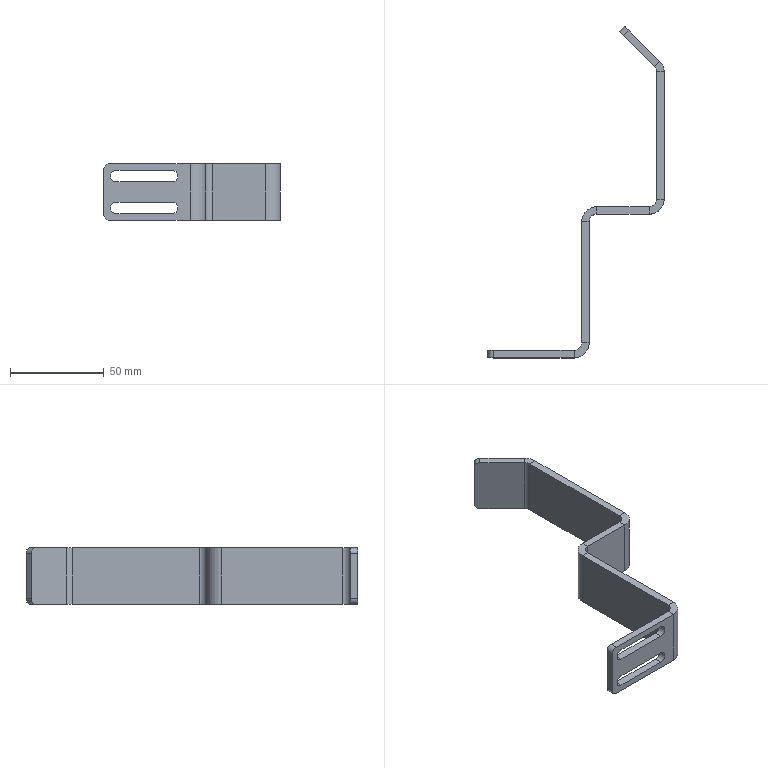Part | NX | features BREP 1 | 1 solid | 50 faces | box 94 x 176.828 x 30 mm | volume 30218 mm3 | plane 34 | cylinder 16 | commonest cylinder face diameters 6 x8 8 x4 16 x4
STEP:
#1=CARTESIAN_POINT('',(-32.,72.57,30.));
#2=VERTEX_POINT('',#1);
#3=CARTESIAN_POINT('',(-4.,72.57,30.));
#4=VERTEX_POINT('',#3);
#5=CARTESIAN_POINT('',(-75.773,72.57,30.));
#6=DIRECTION('',(1.,0.,0.));
#7=VECTOR('',#6,1000.);
#8=LINE('',#5,#7);
#9=EDGE_CURVE('',#2,#4,#8,.T.);
#10=ORIENTED_EDGE('',*,*,#9,.F.);
#11=CARTESIAN_POINT('',(-32.,72.57,0.));
#12=VERTEX_POINT('',#11);
#13=CARTESIAN_POINT('',(-32.,72.57,30.));
#14=DIRECTION('',(0.,0.,-1.));
#15=VECTOR('',#14,1000.);
#16=LINE('',#13,#15);
#17=EDGE_CURVE('',#2,#12,#16,.T.);
#18=ORIENTED_EDGE('',*,*,#17,.T.);
#19=CARTESIAN_POINT('',(-4.,72.57,0.));
#20=VERTEX_POINT('',#19);
#21=CARTESIAN_POINT('',(-75.773,72.57,0.));
#22=DIRECTION('',(1.,0.,0.));
#23=VECTOR('',#22,1000.);
#24=LINE('',#21,#23);
#25=EDGE_CURVE('',#12,#20,#24,.T.);
#26=ORIENTED_EDGE('',*,*,#25,.T.);
#27=CARTESIAN_POINT('',(-4.,72.57,30.));
#28=DIRECTION('',(0.,0.,-1.));
#29=VECTOR('',#28,1000.);
#30=LINE('',#27,#29);
#31=EDGE_CURVE('',#4,#20,#30,.T.);
#32=ORIENTED_EDGE('',*,*,#31,.F.);
#33=EDGE_LOOP('',(#10,#18,#26,#32));
#34=FACE_BOUND('',#33,.T.);
#35=CARTESIAN_POINT('',(-75.773,72.57,30.));
#36=DIRECTION('',(0.,1.,0.));
#37=DIRECTION('',(0.,0.,-1.));
#38=AXIS2_PLACEMENT_3D('',#35,#36,#37);
#39=PLANE('',#38);
#40=ADVANCED_FACE('',(#34),#39,.F.);
#41=CARTESIAN_POINT('',(-32.,76.57,30.));
#42=VERTEX_POINT('',#41);
#43=CARTESIAN_POINT('',(-32.,76.57,0.));
#44=VERTEX_POINT('',#43);
#45=CARTESIAN_POINT('',(-32.,76.57,30.));
#46=DIRECTION('',(0.,0.,-1.));
#47=VECTOR('',#46,1000.);
#48=LINE('',#45,#47);
#49=EDGE_CURVE('',#42,#44,#48,.T.);
#50=ORIENTED_EDGE('',*,*,#49,.F.);
#51=CARTESIAN_POINT('',(-4.,76.57,30.));
#52=VERTEX_POINT('',#51);
#53=CARTESIAN_POINT('',(-75.773,76.57,30.));
#54=DIRECTION('',(1.,0.,0.));
#55=VECTOR('',#54,1000.);
#56=LINE('',#53,#55);
#57=EDGE_CURVE('',#42,#52,#56,.T.);
#58=ORIENTED_EDGE('',*,*,#57,.T.);
#59=CARTESIAN_POINT('',(-4.,76.57,0.));
#60=VERTEX_POINT('',#59);
#61=CARTESIAN_POINT('',(-4.,76.57,30.));
#62=DIRECTION('',(0.,0.,-1.));
#63=VECTOR('',#62,1000.);
#64=LINE('',#61,#63);
#65=EDGE_CURVE('',#52,#60,#64,.T.);
#66=ORIENTED_EDGE('',*,*,#65,.T.);
#67=CARTESIAN_POINT('',(-75.773,76.57,0.));
#68=DIRECTION('',(1.,0.,0.));
#69=VECTOR('',#68,1000.);
#70=LINE('',#67,#69);
#71=EDGE_CURVE('',#44,#60,#70,.T.);
#72=ORIENTED_EDGE('',*,*,#71,.F.);
#73=EDGE_LOOP('',(#50,#58,#66,#72));
#74=FACE_BOUND('',#73,.T.);
#75=CARTESIAN_POINT('',(-75.773,76.57,30.));
#76=DIRECTION('',(0.,1.,0.));
#77=DIRECTION('',(0.,0.,-1.));
#78=AXIS2_PLACEMENT_3D('',#75,#76,#77);
#79=PLANE('',#78);
#80=ADVANCED_FACE('',(#74),#79,.T.);
#81=CARTESIAN_POINT('',(-32.,74.913,0.));
#82=DIRECTION('',(0.,-1.,0.));
#83=VECTOR('',#82,1000.);
#84=LINE('',#81,#83);
#85=EDGE_CURVE('',#44,#12,#84,.T.);
#86=ORIENTED_EDGE('',*,*,#85,.F.);
#87=ORIENTED_EDGE('',*,*,#71,.T.);
#88=CARTESIAN_POINT('',(-4.,74.913,0.));
#89=DIRECTION('',(0.,-1.,0.));
#90=VECTOR('',#89,1000.);
#91=LINE('',#88,#90);
#92=EDGE_CURVE('',#60,#20,#91,.T.);
#93=ORIENTED_EDGE('',*,*,#92,.T.);
#94=ORIENTED_EDGE('',*,*,#25,.F.);
#95=EDGE_LOOP('',(#86,#87,#93,#94));
#96=FACE_BOUND('',#95,.T.);
#97=CARTESIAN_POINT('',(78.227,74.913,0.));
#98=DIRECTION('',(0.,0.,-1.));
#99=DIRECTION('',(0.,-1.,0.));
#100=AXIS2_PLACEMENT_3D('',#97,#98,#99);
#101=PLANE('',#100);
#102=ADVANCED_FACE('',(#96),#101,.T.);
#103=CARTESIAN_POINT('',(-32.,80.57,30.));
#104=DIRECTION('',(0.,1.,0.));
#105=VECTOR('',#104,1000.);
#106=LINE('',#103,#105);
#107=EDGE_CURVE('',#2,#42,#106,.T.);
#108=ORIENTED_EDGE('',*,*,#107,.F.);
#109=ORIENTED_EDGE('',*,*,#9,.T.);
#110=CARTESIAN_POINT('',(-4.,80.57,30.));
#111=DIRECTION('',(0.,1.,0.));
#112=VECTOR('',#111,1000.);
#113=LINE('',#110,#112);
#114=EDGE_CURVE('',#4,#52,#113,.T.);
#115=ORIENTED_EDGE('',*,*,#114,.T.);
#116=ORIENTED_EDGE('',*,*,#57,.F.);
#117=EDGE_LOOP('',(#108,#109,#115,#116));
#118=FACE_BOUND('',#117,.T.);
#119=CARTESIAN_POINT('',(-79.773,80.57,30.));
#120=DIRECTION('',(0.,0.,1.));
#121=DIRECTION('',(0.,1.,0.));
#122=AXIS2_PLACEMENT_3D('',#119,#120,#121);
#123=PLANE('',#122);
#124=ADVANCED_FACE('',(#118),#123,.T.);
#125=CARTESIAN_POINT('',(-17.172,172.828,27.));
#126=VERTEX_POINT('',#125);
#127=CARTESIAN_POINT('',(-17.172,172.828,3.));
#128=VERTEX_POINT('',#127);
#129=CARTESIAN_POINT('',(-17.172,172.828,30.));
#130=DIRECTION('',(0.,0.,-1.));
#131=VECTOR('',#130,1000.);
#132=LINE('',#129,#131);
#133=EDGE_CURVE('',#126,#128,#132,.T.);
#134=ORIENTED_EDGE('',*,*,#133,.T.);
#135=CARTESIAN_POINT('',(-20.,170.,3.));
#136=VERTEX_POINT('',#135);
#137=CARTESIAN_POINT('',(-20.,170.,3.));
#138=DIRECTION('',(-0.7071,-0.7071,0.));
#139=VECTOR('',#138,1000.);
#140=LINE('',#137,#139);
#141=EDGE_CURVE('',#128,#136,#140,.T.);
#142=ORIENTED_EDGE('',*,*,#141,.T.);
#143=CARTESIAN_POINT('',(-20.,170.,27.));
#144=VERTEX_POINT('',#143);
#145=CARTESIAN_POINT('',(-20.,170.,30.));
#146=DIRECTION('',(0.,0.,-1.));
#147=VECTOR('',#146,1000.);
#148=LINE('',#145,#147);
#149=EDGE_CURVE('',#144,#136,#148,.T.);
#150=ORIENTED_EDGE('',*,*,#149,.F.);
#151=CARTESIAN_POINT('',(-20.,170.,27.));
#152=DIRECTION('',(0.7071,0.7071,0.));
#153=VECTOR('',#152,1000.);
#154=LINE('',#151,#153);
#155=EDGE_CURVE('',#144,#126,#154,.T.);
#156=ORIENTED_EDGE('',*,*,#155,.T.);
#157=EDGE_LOOP('',(#134,#142,#150,#156));
#158=FACE_BOUND('',#157,.T.);
#159=CARTESIAN_POINT('',(-20.,170.,30.));
#160=DIRECTION('',(-0.7071,0.7071,0.));
#161=DIRECTION('',(0.7071,0.7071,0.));
#162=AXIS2_PLACEMENT_3D('',#159,#160,#161);
#163=PLANE('',#162);
#164=ADVANCED_FACE('',(#158),#163,.T.);
#165=CARTESIAN_POINT('',(-1.172,151.172,0.));
#166=VERTEX_POINT('',#165);
#167=CARTESIAN_POINT('',(-17.879,167.879,0.));
#168=VERTEX_POINT('',#167);
#169=CARTESIAN_POINT('',(0.,150.,0.));
#170=DIRECTION('',(-0.7071,0.7071,0.));
#171=VECTOR('',#170,1000.);
#172=LINE('',#169,#171);
#173=EDGE_CURVE('',#166,#168,#172,.T.);
#174=ORIENTED_EDGE('',*,*,#173,.T.);
#175=CARTESIAN_POINT('',(-15.05,170.707,0.));
#176=VERTEX_POINT('',#175);
#177=CARTESIAN_POINT('',(-20.707,165.05,0.));
#178=DIRECTION('',(0.7071,0.7071,0.));
#179=VECTOR('',#178,1000.);
#180=LINE('',#177,#179);
#181=EDGE_CURVE('',#168,#176,#180,.T.);
#182=ORIENTED_EDGE('',*,*,#181,.T.);
#183=CARTESIAN_POINT('',(1.657,154.,0.));
#184=VERTEX_POINT('',#183);
#185=CARTESIAN_POINT('',(2.828,152.828,0.));
#186=DIRECTION('',(-0.7071,0.7071,0.));
#187=VECTOR('',#186,1000.);
#188=LINE('',#185,#187);
#189=EDGE_CURVE('',#184,#176,#188,.T.);
#190=ORIENTED_EDGE('',*,*,#189,.F.);
#191=CARTESIAN_POINT('',(1.657,154.,0.));
#192=DIRECTION('',(-0.7071,-0.7071,0.));
#193=VECTOR('',#192,1000.);
#194=LINE('',#191,#193);
#195=EDGE_CURVE('',#184,#166,#194,.T.);
#196=ORIENTED_EDGE('',*,*,#195,.T.);
#197=EDGE_LOOP('',(#174,#182,#190,#196));
#198=FACE_BOUND('',#197,.T.);
#199=CARTESIAN_POINT('',(-4.,148.343,0.));
#200=DIRECTION('',(0.,0.,-1.));
#201=DIRECTION('',(1.,0.,0.));
#202=AXIS2_PLACEMENT_3D('',#199,#200,#201);
#203=PLANE('',#202);
#204=ADVANCED_FACE('',(#198),#203,.T.);
#205=ORIENTED_EDGE('',*,*,#189,.T.);
#206=CARTESIAN_POINT('',(-15.05,170.707,3.));
#207=DIRECTION('',(0.7071,0.7071,0.));
#208=DIRECTION('',(0.7071,-0.7071,0.));
#209=AXIS2_PLACEMENT_3D('',#206,#207,#208);
#210=CIRCLE('',#209,3.);
#211=EDGE_CURVE('',#176,#128,#210,.T.);
#212=ORIENTED_EDGE('',*,*,#211,.T.);
#213=ORIENTED_EDGE('',*,*,#133,.F.);
#214=CARTESIAN_POINT('',(-15.05,170.707,30.));
#215=VERTEX_POINT('',#214);
#216=CARTESIAN_POINT('',(-15.05,170.707,27.));
#217=DIRECTION('',(0.7071,0.7071,0.));
#218=DIRECTION('',(0.7071,-0.7071,0.));
#219=AXIS2_PLACEMENT_3D('',#216,#217,#218);
#220=CIRCLE('',#219,3.);
#221=EDGE_CURVE('',#126,#215,#220,.T.);
#222=ORIENTED_EDGE('',*,*,#221,.T.);
#223=CARTESIAN_POINT('',(1.657,154.,30.));
#224=VERTEX_POINT('',#223);
#225=CARTESIAN_POINT('',(2.828,152.828,30.));
#226=DIRECTION('',(-0.7071,0.7071,0.));
#227=VECTOR('',#226,1000.);
#228=LINE('',#225,#227);
#229=EDGE_CURVE('',#224,#215,#228,.T.);
#230=ORIENTED_EDGE('',*,*,#229,.F.);
#231=CARTESIAN_POINT('',(1.657,154.,30.));
#232=DIRECTION('',(0.,0.,-1.));
#233=VECTOR('',#232,1000.);
#234=LINE('',#231,#233);
#235=EDGE_CURVE('',#224,#184,#234,.T.);
#236=ORIENTED_EDGE('',*,*,#235,.T.);
#237=EDGE_LOOP('',(#205,#212,#213,#222,#230,#236));
#238=FACE_BOUND('',#237,.T.);
#239=CARTESIAN_POINT('',(2.828,152.828,30.));
#240=DIRECTION('',(-0.7071,-0.7071,0.));
#241=DIRECTION('',(-0.7071,0.7071,0.));
#242=AXIS2_PLACEMENT_3D('',#239,#240,#241);
#243=PLANE('',#242);
#244=ADVANCED_FACE('',(#238),#243,.F.);
#245=ORIENTED_EDGE('',*,*,#229,.T.);
#246=CARTESIAN_POINT('',(-17.879,167.879,30.));
#247=VERTEX_POINT('',#246);
#248=CARTESIAN_POINT('',(-16.707,169.05,30.));
#249=DIRECTION('',(-0.7071,-0.7071,0.));
#250=VECTOR('',#249,1000.);
#251=LINE('',#248,#250);
#252=EDGE_CURVE('',#215,#247,#251,.T.);
#253=ORIENTED_EDGE('',*,*,#252,.T.);
#254=CARTESIAN_POINT('',(-1.172,151.172,30.));
#255=VERTEX_POINT('',#254);
#256=CARTESIAN_POINT('',(0.,150.,30.));
#257=DIRECTION('',(-0.7071,0.7071,0.));
#258=VECTOR('',#257,1000.);
#259=LINE('',#256,#258);
#260=EDGE_CURVE('',#255,#247,#259,.T.);
#261=ORIENTED_EDGE('',*,*,#260,.F.);
#262=CARTESIAN_POINT('',(-1.172,151.172,30.));
#263=DIRECTION('',(0.7071,0.7071,0.));
#264=VECTOR('',#263,1000.);
#265=LINE('',#262,#264);
#266=EDGE_CURVE('',#255,#224,#265,.T.);
#267=ORIENTED_EDGE('',*,*,#266,.T.);
#268=EDGE_LOOP('',(#245,#253,#261,#267));
#269=FACE_BOUND('',#268,.T.);
#270=CARTESIAN_POINT('',(4.,148.343,30.));
#271=DIRECTION('',(0.,0.,1.));
#272=DIRECTION('',(-1.,0.,0.));
#273=AXIS2_PLACEMENT_3D('',#270,#271,#272);
#274=PLANE('',#273);
#275=ADVANCED_FACE('',(#269),#274,.T.);
#276=ORIENTED_EDGE('',*,*,#149,.T.);
#277=CARTESIAN_POINT('',(-17.879,167.879,3.));
#278=DIRECTION('',(-0.7071,-0.7071,0.));
#279=DIRECTION('',(0.7071,-0.7071,0.));
#280=AXIS2_PLACEMENT_3D('',#277,#278,#279);
#281=CIRCLE('',#280,3.);
#282=EDGE_CURVE('',#136,#168,#281,.T.);
#283=ORIENTED_EDGE('',*,*,#282,.T.);
#284=ORIENTED_EDGE('',*,*,#173,.F.);
#285=CARTESIAN_POINT('',(-1.172,151.172,30.));
#286=DIRECTION('',(0.,0.,-1.));
#287=VECTOR('',#286,1000.);
#288=LINE('',#285,#287);
#289=EDGE_CURVE('',#255,#166,#288,.T.);
#290=ORIENTED_EDGE('',*,*,#289,.F.);
#291=ORIENTED_EDGE('',*,*,#260,.T.);
#292=CARTESIAN_POINT('',(-17.879,167.879,27.));
#293=DIRECTION('',(-0.7071,-0.7071,0.));
#294=DIRECTION('',(0.7071,-0.7071,0.));
#295=AXIS2_PLACEMENT_3D('',#292,#293,#294);
#296=CIRCLE('',#295,3.);
#297=EDGE_CURVE('',#247,#144,#296,.T.);
#298=ORIENTED_EDGE('',*,*,#297,.T.);
#299=EDGE_LOOP('',(#276,#283,#284,#290,#291,#298));
#300=FACE_BOUND('',#299,.T.);
#301=CARTESIAN_POINT('',(0.,150.,30.));
#302=DIRECTION('',(-0.7071,-0.7071,0.));
#303=DIRECTION('',(-0.7071,0.7071,0.));
#304=AXIS2_PLACEMENT_3D('',#301,#302,#303);
#305=PLANE('',#304);
#306=ADVANCED_FACE('',(#300),#305,.T.);
#307=CARTESIAN_POINT('',(0.,148.343,0.));
#308=VERTEX_POINT('',#307);
#309=CARTESIAN_POINT('',(4.,148.343,0.));
#310=VERTEX_POINT('',#309);
#311=CARTESIAN_POINT('',(0.,148.343,0.));
#312=DIRECTION('',(1.,0.,0.));
#313=VECTOR('',#312,1000.);
#314=LINE('',#311,#313);
#315=EDGE_CURVE('',#308,#310,#314,.T.);
#316=ORIENTED_EDGE('',*,*,#315,.F.);
#317=CARTESIAN_POINT('',(-4.,148.343,0.));
#318=DIRECTION('',(0.,0.,1.));
#319=DIRECTION('',(-1.,0.,0.));
#320=AXIS2_PLACEMENT_3D('',#317,#318,#319);
#321=CIRCLE('',#320,4.);
#322=EDGE_CURVE('',#308,#166,#321,.T.);
#323=ORIENTED_EDGE('',*,*,#322,.T.);
#324=ORIENTED_EDGE('',*,*,#195,.F.);
#325=CARTESIAN_POINT('',(-4.,148.343,0.));
#326=DIRECTION('',(0.,0.,1.));
#327=DIRECTION('',(1.,0.,0.));
#328=AXIS2_PLACEMENT_3D('',#325,#326,#327);
#329=CIRCLE('',#328,8.);
#330=EDGE_CURVE('',#310,#184,#329,.T.);
#331=ORIENTED_EDGE('',*,*,#330,.F.);
#332=EDGE_LOOP('',(#316,#323,#324,#331));
#333=FACE_BOUND('',#332,.T.);
#334=CARTESIAN_POINT('',(0.,148.343,0.));
#335=DIRECTION('',(0.,0.,-1.));
#336=DIRECTION('',(1.,0.,0.));
#337=AXIS2_PLACEMENT_3D('',#334,#335,#336);
#338=PLANE('',#337);
#339=ADVANCED_FACE('',(#333),#338,.T.);
#340=ORIENTED_EDGE('',*,*,#330,.T.);
#341=ORIENTED_EDGE('',*,*,#235,.F.);
#342=CARTESIAN_POINT('',(4.,148.343,30.));
#343=VERTEX_POINT('',#342);
#344=CARTESIAN_POINT('',(-4.,148.343,30.));
#345=DIRECTION('',(0.,0.,1.));
#346=DIRECTION('',(1.,0.,0.));
#347=AXIS2_PLACEMENT_3D('',#344,#345,#346);
#348=CIRCLE('',#347,8.);
#349=EDGE_CURVE('',#343,#224,#348,.T.);
#350=ORIENTED_EDGE('',*,*,#349,.F.);
#351=CARTESIAN_POINT('',(4.,148.343,30.));
#352=DIRECTION('',(0.,0.,-1.));
#353=VECTOR('',#352,1000.);
#354=LINE('',#351,#353);
#355=EDGE_CURVE('',#343,#310,#354,.T.);
#356=ORIENTED_EDGE('',*,*,#355,.T.);
#357=EDGE_LOOP('',(#340,#341,#350,#356));
#358=FACE_BOUND('',#357,.T.);
#359=CARTESIAN_POINT('',(-4.,148.343,30.));
#360=DIRECTION('',(0.,0.,-1.));
#361=DIRECTION('',(1.,0.,0.));
#362=AXIS2_PLACEMENT_3D('',#359,#360,#361);
#363=CYLINDRICAL_SURFACE('',#362,8.);
#364=ADVANCED_FACE('',(#358),#363,.T.);
#365=ORIENTED_EDGE('',*,*,#266,.F.);
#366=CARTESIAN_POINT('',(0.,148.343,30.));
#367=VERTEX_POINT('',#366);
#368=CARTESIAN_POINT('',(-4.,148.343,30.));
#369=DIRECTION('',(0.,0.,1.));
#370=DIRECTION('',(-1.,0.,0.));
#371=AXIS2_PLACEMENT_3D('',#368,#369,#370);
#372=CIRCLE('',#371,4.);
#373=EDGE_CURVE('',#367,#255,#372,.T.);
#374=ORIENTED_EDGE('',*,*,#373,.F.);
#375=CARTESIAN_POINT('',(4.,148.343,30.));
#376=DIRECTION('',(-1.,0.,0.));
#377=VECTOR('',#376,1000.);
#378=LINE('',#375,#377);
#379=EDGE_CURVE('',#343,#367,#378,.T.);
#380=ORIENTED_EDGE('',*,*,#379,.F.);
#381=ORIENTED_EDGE('',*,*,#349,.T.);
#382=EDGE_LOOP('',(#365,#374,#380,#381));
#383=FACE_BOUND('',#382,.T.);
#384=CARTESIAN_POINT('',(-1.172,151.172,30.));
#385=DIRECTION('',(0.,0.,1.));
#386=DIRECTION('',(-1.,0.,0.));
#387=AXIS2_PLACEMENT_3D('',#384,#385,#386);
#388=PLANE('',#387);
#389=ADVANCED_FACE('',(#383),#388,.T.);
#390=ORIENTED_EDGE('',*,*,#322,.F.);
#391=CARTESIAN_POINT('',(0.,148.343,30.));
#392=DIRECTION('',(0.,0.,-1.));
#393=VECTOR('',#392,1000.);
#394=LINE('',#391,#393);
#395=EDGE_CURVE('',#367,#308,#394,.T.);
#396=ORIENTED_EDGE('',*,*,#395,.F.);
#397=ORIENTED_EDGE('',*,*,#373,.T.);
#398=ORIENTED_EDGE('',*,*,#289,.T.);
#399=EDGE_LOOP('',(#390,#396,#397,#398));
#400=FACE_BOUND('',#399,.T.);
#401=CARTESIAN_POINT('',(-4.,148.343,30.));
#402=DIRECTION('',(0.,0.,-1.));
#403=DIRECTION('',(1.,0.,0.));
#404=AXIS2_PLACEMENT_3D('',#401,#402,#403);
#405=CYLINDRICAL_SURFACE('',#404,4.);
#406=ADVANCED_FACE('',(#400),#405,.F.);
#407=CARTESIAN_POINT('',(0.,80.57,30.));
#408=VERTEX_POINT('',#407);
#409=CARTESIAN_POINT('',(0.,80.57,0.));
#410=VERTEX_POINT('',#409);
#411=CARTESIAN_POINT('',(0.,80.57,30.));
#412=DIRECTION('',(0.,0.,-1.));
#413=VECTOR('',#412,1000.);
#414=LINE('',#411,#413);
#415=EDGE_CURVE('',#408,#410,#414,.T.);
#416=ORIENTED_EDGE('',*,*,#415,.F.);
#417=CARTESIAN_POINT('',(0.,0.,30.));
#418=DIRECTION('',(0.,1.,0.));
#419=VECTOR('',#418,1000.);
#420=LINE('',#417,#419);
#421=EDGE_CURVE('',#408,#367,#420,.T.);
#422=ORIENTED_EDGE('',*,*,#421,.T.);
#423=ORIENTED_EDGE('',*,*,#395,.T.);
#424=CARTESIAN_POINT('',(0.,0.,0.));
#425=DIRECTION('',(0.,1.,0.));
#426=VECTOR('',#425,1000.);
#427=LINE('',#424,#426);
#428=EDGE_CURVE('',#410,#308,#427,.T.);
#429=ORIENTED_EDGE('',*,*,#428,.F.);
#430=EDGE_LOOP('',(#416,#422,#423,#429));
#431=FACE_BOUND('',#430,.T.);
#432=CARTESIAN_POINT('',(0.,0.,30.));
#433=DIRECTION('',(-1.,0.,0.));
#434=DIRECTION('',(0.,0.,-1.));
#435=AXIS2_PLACEMENT_3D('',#432,#433,#434);
#436=PLANE('',#435);
#437=ADVANCED_FACE('',(#431),#436,.T.);
#438=CARTESIAN_POINT('',(4.,80.57,30.));
#439=VERTEX_POINT('',#438);
#440=CARTESIAN_POINT('',(-4.,80.57,30.));
#441=DIRECTION('',(-1.,0.,0.));
#442=VECTOR('',#441,1000.);
#443=LINE('',#440,#442);
#444=EDGE_CURVE('',#439,#408,#443,.T.);
#445=ORIENTED_EDGE('',*,*,#444,.F.);
#446=CARTESIAN_POINT('',(4.,0.,30.));
#447=DIRECTION('',(0.,1.,0.));
#448=VECTOR('',#447,1000.);
#449=LINE('',#446,#448);
#450=EDGE_CURVE('',#439,#343,#449,.T.);
#451=ORIENTED_EDGE('',*,*,#450,.T.);
#452=ORIENTED_EDGE('',*,*,#379,.T.);
#453=ORIENTED_EDGE('',*,*,#421,.F.);
#454=EDGE_LOOP('',(#445,#451,#452,#453));
#455=FACE_BOUND('',#454,.T.);
#456=CARTESIAN_POINT('',(-4.,-4.,30.));
#457=DIRECTION('',(0.,0.,1.));
#458=DIRECTION('',(-1.,0.,0.));
#459=AXIS2_PLACEMENT_3D('',#456,#457,#458);
#460=PLANE('',#459);
#461=ADVANCED_FACE('',(#455),#460,.T.);
#462=ORIENTED_EDGE('',*,*,#450,.F.);
#463=CARTESIAN_POINT('',(4.,80.57,0.));
#464=VERTEX_POINT('',#463);
#465=CARTESIAN_POINT('',(4.,80.57,30.));
#466=DIRECTION('',(0.,0.,-1.));
#467=VECTOR('',#466,1000.);
#468=LINE('',#465,#467);
#469=EDGE_CURVE('',#439,#464,#468,.T.);
#470=ORIENTED_EDGE('',*,*,#469,.T.);
#471=CARTESIAN_POINT('',(4.,0.,0.));
#472=DIRECTION('',(0.,1.,0.));
#473=VECTOR('',#472,1000.);
#474=LINE('',#471,#473);
#475=EDGE_CURVE('',#464,#310,#474,.T.);
#476=ORIENTED_EDGE('',*,*,#475,.T.);
#477=ORIENTED_EDGE('',*,*,#355,.F.);
#478=EDGE_LOOP('',(#462,#470,#476,#477));
#479=FACE_BOUND('',#478,.T.);
#480=CARTESIAN_POINT('',(4.,0.,30.));
#481=DIRECTION('',(-1.,0.,0.));
#482=DIRECTION('',(0.,0.,-1.));
#483=AXIS2_PLACEMENT_3D('',#480,#481,#482);
#484=PLANE('',#483);
#485=ADVANCED_FACE('',(#479),#484,.F.);
#486=CARTESIAN_POINT('',(1.657,80.57,0.));
#487=DIRECTION('',(1.,0.,0.));
#488=VECTOR('',#487,1000.);
#489=LINE('',#486,#488);
#490=EDGE_CURVE('',#410,#464,#489,.T.);
#491=ORIENTED_EDGE('',*,*,#490,.F.);
#492=ORIENTED_EDGE('',*,*,#428,.T.);
#493=ORIENTED_EDGE('',*,*,#315,.T.);
#494=ORIENTED_EDGE('',*,*,#475,.F.);
#495=EDGE_LOOP('',(#491,#492,#493,#494));
#496=FACE_BOUND('',#495,.T.);
#497=CARTESIAN_POINT('',(1.657,154.,0.));
#498=DIRECTION('',(0.,0.,-1.));
#499=DIRECTION('',(1.,0.,0.));
#500=AXIS2_PLACEMENT_3D('',#497,#498,#499);
#501=PLANE('',#500);
#502=ADVANCED_FACE('',(#496),#501,.T.);
#503=ORIENTED_EDGE('',*,*,#114,.F.);
#504=CARTESIAN_POINT('',(-4.,80.57,30.));
#505=DIRECTION('',(0.,0.,1.));
#506=DIRECTION('',(1.,0.,0.));
#507=AXIS2_PLACEMENT_3D('',#504,#505,#506);
#508=CIRCLE('',#507,8.);
#509=EDGE_CURVE('',#4,#439,#508,.T.);
#510=ORIENTED_EDGE('',*,*,#509,.T.);
#511=ORIENTED_EDGE('',*,*,#444,.T.);
#512=CARTESIAN_POINT('',(-4.,80.57,30.));
#513=DIRECTION('',(0.,0.,1.));
#514=DIRECTION('',(1.,0.,0.));
#515=AXIS2_PLACEMENT_3D('',#512,#513,#514);
#516=CIRCLE('',#515,4.);
#517=EDGE_CURVE('',#52,#408,#516,.T.);
#518=ORIENTED_EDGE('',*,*,#517,.F.);
#519=EDGE_LOOP('',(#503,#510,#511,#518));
#520=FACE_BOUND('',#519,.T.);
#521=CARTESIAN_POINT('',(-4.,80.57,30.));
#522=DIRECTION('',(0.,0.,-1.));
#523=DIRECTION('',(1.,0.,0.));
#524=AXIS2_PLACEMENT_3D('',#521,#522,#523);
#525=PLANE('',#524);
#526=ADVANCED_FACE('',(#520),#525,.F.);
#527=CARTESIAN_POINT('',(-4.,80.57,0.));
#528=DIRECTION('',(0.,0.,-1.));
#529=DIRECTION('',(1.,0.,0.));
#530=AXIS2_PLACEMENT_3D('',#527,#528,#529);
#531=CIRCLE('',#530,8.);
#532=EDGE_CURVE('',#464,#20,#531,.T.);
#533=ORIENTED_EDGE('',*,*,#532,.T.);
#534=ORIENTED_EDGE('',*,*,#92,.F.);
#535=CARTESIAN_POINT('',(-4.,80.57,0.));
#536=DIRECTION('',(0.,0.,-1.));
#537=DIRECTION('',(1.,0.,0.));
#538=AXIS2_PLACEMENT_3D('',#535,#536,#537);
#539=CIRCLE('',#538,4.);
#540=EDGE_CURVE('',#410,#60,#539,.T.);
#541=ORIENTED_EDGE('',*,*,#540,.F.);
#542=ORIENTED_EDGE('',*,*,#490,.T.);
#543=EDGE_LOOP('',(#533,#534,#541,#542));
#544=FACE_BOUND('',#543,.T.);
#545=CARTESIAN_POINT('',(-4.,80.57,0.));
#546=DIRECTION('',(0.,0.,1.));
#547=DIRECTION('',(-1.,0.,0.));
#548=AXIS2_PLACEMENT_3D('',#545,#546,#547);
#549=PLANE('',#548);
#550=ADVANCED_FACE('',(#544),#549,.F.);
#551=ORIENTED_EDGE('',*,*,#415,.T.);
#552=ORIENTED_EDGE('',*,*,#540,.T.);
#553=ORIENTED_EDGE('',*,*,#65,.F.);
#554=ORIENTED_EDGE('',*,*,#517,.T.);
#555=EDGE_LOOP('',(#551,#552,#553,#554));
#556=FACE_BOUND('',#555,.T.);
#557=CARTESIAN_POINT('',(-4.,80.57,-16.518));
#558=DIRECTION('',(0.,0.,1.));
#559=DIRECTION('',(-1.,0.,0.));
#560=AXIS2_PLACEMENT_3D('',#557,#558,#559);
#561=CYLINDRICAL_SURFACE('',#560,4.);
#562=ADVANCED_FACE('',(#556),#561,.F.);
#563=ORIENTED_EDGE('',*,*,#469,.F.);
#564=ORIENTED_EDGE('',*,*,#509,.F.);
#565=ORIENTED_EDGE('',*,*,#31,.T.);
#566=ORIENTED_EDGE('',*,*,#532,.F.);
#567=EDGE_LOOP('',(#563,#564,#565,#566));
#568=FACE_BOUND('',#567,.T.);
#569=CARTESIAN_POINT('',(-4.,80.57,-16.518));
#570=DIRECTION('',(0.,0.,1.));
#571=DIRECTION('',(-1.,0.,0.));
#572=AXIS2_PLACEMENT_3D('',#569,#570,#571);
#573=CYLINDRICAL_SURFACE('',#572,8.);
#574=ADVANCED_FACE('',(#568),#573,.T.);
#575=CARTESIAN_POINT('',(-36.,68.57,30.));
#576=VERTEX_POINT('',#575);
#577=CARTESIAN_POINT('',(-40.,68.57,30.));
#578=VERTEX_POINT('',#577);
#579=CARTESIAN_POINT('',(-44.,68.57,30.));
#580=DIRECTION('',(-1.,0.,0.));
#581=VECTOR('',#580,1000.);
#582=LINE('',#579,#581);
#583=EDGE_CURVE('',#576,#578,#582,.T.);
#584=ORIENTED_EDGE('',*,*,#583,.F.);
#585=CARTESIAN_POINT('',(-32.,68.57,30.));
#586=DIRECTION('',(0.,0.,-1.));
#587=DIRECTION('',(1.,0.,0.));
#588=AXIS2_PLACEMENT_3D('',#585,#586,#587);
#589=CIRCLE('',#588,4.);
#590=EDGE_CURVE('',#576,#2,#589,.T.);
#591=ORIENTED_EDGE('',*,*,#590,.T.);
#592=ORIENTED_EDGE('',*,*,#107,.T.);
#593=CARTESIAN_POINT('',(-32.,68.57,30.));
#594=DIRECTION('',(0.,0.,-1.));
#595=DIRECTION('',(-1.,0.,0.));
#596=AXIS2_PLACEMENT_3D('',#593,#594,#595);
#597=CIRCLE('',#596,8.);
#598=EDGE_CURVE('',#578,#42,#597,.T.);
#599=ORIENTED_EDGE('',*,*,#598,.F.);
#600=EDGE_LOOP('',(#584,#591,#592,#599));
#601=FACE_BOUND('',#600,.T.);
#602=CARTESIAN_POINT('',(-32.,68.57,30.));
#603=DIRECTION('',(0.,0.,1.));
#604=DIRECTION('',(-1.,0.,0.));
#605=AXIS2_PLACEMENT_3D('',#602,#603,#604);
#606=PLANE('',#605);
#607=ADVANCED_FACE('',(#601),#606,.T.);
#608=CARTESIAN_POINT('',(-36.,68.57,0.));
#609=VERTEX_POINT('',#608);
#610=CARTESIAN_POINT('',(-32.,68.57,0.));
#611=DIRECTION('',(0.,0.,1.));
#612=DIRECTION('',(1.,0.,0.));
#613=AXIS2_PLACEMENT_3D('',#610,#611,#612);
#614=CIRCLE('',#613,4.);
#615=EDGE_CURVE('',#12,#609,#614,.T.);
#616=ORIENTED_EDGE('',*,*,#615,.T.);
#617=CARTESIAN_POINT('',(-40.,68.57,0.));
#618=VERTEX_POINT('',#617);
#619=CARTESIAN_POINT('',(-38.343,68.57,0.));
#620=DIRECTION('',(1.,0.,0.));
#621=VECTOR('',#620,1000.);
#622=LINE('',#619,#621);
#623=EDGE_CURVE('',#618,#609,#622,.T.);
#624=ORIENTED_EDGE('',*,*,#623,.F.);
#625=CARTESIAN_POINT('',(-32.,68.57,0.));
#626=DIRECTION('',(0.,0.,1.));
#627=DIRECTION('',(-1.,0.,0.));
#628=AXIS2_PLACEMENT_3D('',#625,#626,#627);
#629=CIRCLE('',#628,8.);
#630=EDGE_CURVE('',#44,#618,#629,.T.);
#631=ORIENTED_EDGE('',*,*,#630,.F.);
#632=ORIENTED_EDGE('',*,*,#85,.T.);
#633=EDGE_LOOP('',(#616,#624,#631,#632));
#634=FACE_BOUND('',#633,.T.);
#635=CARTESIAN_POINT('',(-32.,68.57,0.));
#636=DIRECTION('',(0.,0.,-1.));
#637=DIRECTION('',(1.,0.,0.));
#638=AXIS2_PLACEMENT_3D('',#635,#636,#637);
#639=PLANE('',#638);
#640=ADVANCED_FACE('',(#634),#639,.T.);
#641=ORIENTED_EDGE('',*,*,#49,.T.);
#642=ORIENTED_EDGE('',*,*,#630,.T.);
#643=CARTESIAN_POINT('',(-40.,68.57,30.));
#644=DIRECTION('',(0.,0.,-1.));
#645=VECTOR('',#644,1000.);
#646=LINE('',#643,#645);
#647=EDGE_CURVE('',#578,#618,#646,.T.);
#648=ORIENTED_EDGE('',*,*,#647,.F.);
#649=ORIENTED_EDGE('',*,*,#598,.T.);
#650=EDGE_LOOP('',(#641,#642,#648,#649));
#651=FACE_BOUND('',#650,.T.);
#652=CARTESIAN_POINT('',(-32.,68.57,-16.518));
#653=DIRECTION('',(0.,0.,1.));
#654=DIRECTION('',(-1.,0.,0.));
#655=AXIS2_PLACEMENT_3D('',#652,#653,#654);
#656=CYLINDRICAL_SURFACE('',#655,8.);
#657=ADVANCED_FACE('',(#651),#656,.T.);
#658=ORIENTED_EDGE('',*,*,#17,.F.);
#659=ORIENTED_EDGE('',*,*,#590,.F.);
#660=CARTESIAN_POINT('',(-36.,68.57,30.));
#661=DIRECTION('',(0.,0.,-1.));
#662=VECTOR('',#661,1000.);
#663=LINE('',#660,#662);
#664=EDGE_CURVE('',#576,#609,#663,.T.);
#665=ORIENTED_EDGE('',*,*,#664,.T.);
#666=ORIENTED_EDGE('',*,*,#615,.F.);
#667=EDGE_LOOP('',(#658,#659,#665,#666));
#668=FACE_BOUND('',#667,.T.);
#669=CARTESIAN_POINT('',(-32.,68.57,-16.518));
#670=DIRECTION('',(0.,0.,1.));
#671=DIRECTION('',(-1.,0.,0.));
#672=AXIS2_PLACEMENT_3D('',#669,#670,#671);
#673=CYLINDRICAL_SURFACE('',#672,4.);
#674=ADVANCED_FACE('',(#668),#673,.F.);
#675=CARTESIAN_POINT('',(-90.,0.,27.));
#676=VERTEX_POINT('',#675);
#677=CARTESIAN_POINT('',(-90.,0.,3.));
#678=VERTEX_POINT('',#677);
#679=CARTESIAN_POINT('',(-90.,0.,30.));
#680=DIRECTION('',(0.,0.,-1.));
#681=VECTOR('',#680,1000.);
#682=LINE('',#679,#681);
#683=EDGE_CURVE('',#676,#678,#682,.T.);
#684=ORIENTED_EDGE('',*,*,#683,.T.);
#685=CARTESIAN_POINT('',(-90.,-4.,3.));
#686=VERTEX_POINT('',#685);
#687=CARTESIAN_POINT('',(-90.,-4.,3.));
#688=DIRECTION('',(0.,-1.,0.));
#689=VECTOR('',#688,1000.);
#690=LINE('',#687,#689);
#691=EDGE_CURVE('',#678,#686,#690,.T.);
#692=ORIENTED_EDGE('',*,*,#691,.T.);
#693=CARTESIAN_POINT('',(-90.,-4.,27.));
#694=VERTEX_POINT('',#693);
#695=CARTESIAN_POINT('',(-90.,-4.,30.));
#696=DIRECTION('',(0.,0.,-1.));
#697=VECTOR('',#696,1000.);
#698=LINE('',#695,#697);
#699=EDGE_CURVE('',#694,#686,#698,.T.);
#700=ORIENTED_EDGE('',*,*,#699,.F.);
#701=CARTESIAN_POINT('',(-90.,0.,27.));
#702=DIRECTION('',(0.,1.,0.));
#703=VECTOR('',#702,1000.);
#704=LINE('',#701,#703);
#705=EDGE_CURVE('',#694,#676,#704,.T.);
#706=ORIENTED_EDGE('',*,*,#705,.T.);
#707=EDGE_LOOP('',(#684,#692,#700,#706));
#708=FACE_BOUND('',#707,.T.);
#709=CARTESIAN_POINT('',(-90.,-4.,30.));
#710=DIRECTION('',(-1.,0.,0.));
#711=DIRECTION('',(0.,0.,-1.));
#712=AXIS2_PLACEMENT_3D('',#709,#710,#711);
#713=PLANE('',#712);
#714=ADVANCED_FACE('',(#708),#713,.T.);
#715=CARTESIAN_POINT('',(-87.,0.,30.));
#716=VERTEX_POINT('',#715);
#717=CARTESIAN_POINT('',(-44.,0.,30.));
#718=VERTEX_POINT('',#717);
#719=CARTESIAN_POINT('',(-90.,0.,30.));
#720=DIRECTION('',(1.,0.,0.));
#721=VECTOR('',#720,1000.);
#722=LINE('',#719,#721);
#723=EDGE_CURVE('',#716,#718,#722,.T.);
#724=ORIENTED_EDGE('',*,*,#723,.F.);
#725=CARTESIAN_POINT('',(-87.,-4.,30.));
#726=VERTEX_POINT('',#725);
#727=CARTESIAN_POINT('',(-87.,-4.,30.));
#728=DIRECTION('',(0.,-1.,0.));
#729=VECTOR('',#728,1000.);
#730=LINE('',#727,#729);
#731=EDGE_CURVE('',#716,#726,#730,.T.);
#732=ORIENTED_EDGE('',*,*,#731,.T.);
#733=CARTESIAN_POINT('',(-44.,-4.,30.));
#734=VERTEX_POINT('',#733);
#735=CARTESIAN_POINT('',(-90.,-4.,30.));
#736=DIRECTION('',(1.,0.,0.));
#737=VECTOR('',#736,1000.);
#738=LINE('',#735,#737);
#739=EDGE_CURVE('',#726,#734,#738,.T.);
#740=ORIENTED_EDGE('',*,*,#739,.T.);
#741=CARTESIAN_POINT('',(-44.,-4.,30.));
#742=DIRECTION('',(0.,1.,0.));
#743=VECTOR('',#742,1000.);
#744=LINE('',#741,#743);
#745=EDGE_CURVE('',#734,#718,#744,.T.);
#746=ORIENTED_EDGE('',*,*,#745,.T.);
#747=EDGE_LOOP('',(#724,#732,#740,#746));
#748=FACE_BOUND('',#747,.T.);
#749=CARTESIAN_POINT('',(-44.,148.343,30.));
#750=DIRECTION('',(0.,0.,-1.));
#751=DIRECTION('',(1.,0.,0.));
#752=AXIS2_PLACEMENT_3D('',#749,#750,#751);
#753=PLANE('',#752);
#754=ADVANCED_FACE('',(#748),#753,.F.);
#755=CARTESIAN_POINT('',(-53.5,-4.,3.5));
#756=VERTEX_POINT('',#755);
#757=CARTESIAN_POINT('',(-83.5,-4.,3.5));
#758=VERTEX_POINT('',#757);
#759=CARTESIAN_POINT('',(-90.,-4.,3.5));
#760=DIRECTION('',(-1.,0.,0.));
#761=VECTOR('',#760,1000.);
#762=LINE('',#759,#761);
#763=EDGE_CURVE('',#756,#758,#762,.T.);
#764=ORIENTED_EDGE('',*,*,#763,.T.);
#765=CARTESIAN_POINT('',(-83.5,-4.,9.5));
#766=VERTEX_POINT('',#765);
#767=CARTESIAN_POINT('',(-83.5,-4.,6.5));
#768=DIRECTION('',(0.,1.,0.));
#769=DIRECTION('',(0.,0.,1.));
#770=AXIS2_PLACEMENT_3D('',#767,#768,#769);
#771=CIRCLE('',#770,3.);
#772=EDGE_CURVE('',#758,#766,#771,.T.);
#773=ORIENTED_EDGE('',*,*,#772,.T.);
#774=CARTESIAN_POINT('',(-53.5,-4.,9.5));
#775=VERTEX_POINT('',#774);
#776=CARTESIAN_POINT('',(-90.,-4.,9.5));
#777=DIRECTION('',(1.,0.,0.));
#778=VECTOR('',#777,1000.);
#779=LINE('',#776,#778);
#780=EDGE_CURVE('',#766,#775,#779,.T.);
#781=ORIENTED_EDGE('',*,*,#780,.T.);
#782=CARTESIAN_POINT('',(-53.5,-4.,6.5));
#783=DIRECTION('',(0.,1.,0.));
#784=DIRECTION('',(0.,0.,1.));
#785=AXIS2_PLACEMENT_3D('',#782,#783,#784);
#786=CIRCLE('',#785,3.);
#787=EDGE_CURVE('',#775,#756,#786,.T.);
#788=ORIENTED_EDGE('',*,*,#787,.T.);
#789=EDGE_LOOP('',(#764,#773,#781,#788));
#790=FACE_BOUND('',#789,.T.);
#791=CARTESIAN_POINT('',(-53.5,-4.,20.5));
#792=VERTEX_POINT('',#791);
#793=CARTESIAN_POINT('',(-83.5,-4.,20.5));
#794=VERTEX_POINT('',#793);
#795=CARTESIAN_POINT('',(-90.,-4.,20.5));
#796=DIRECTION('',(-1.,0.,0.));
#797=VECTOR('',#796,1000.);
#798=LINE('',#795,#797);
#799=EDGE_CURVE('',#792,#794,#798,.T.);
#800=ORIENTED_EDGE('',*,*,#799,.T.);
#801=CARTESIAN_POINT('',(-83.5,-4.,26.5));
#802=VERTEX_POINT('',#801);
#803=CARTESIAN_POINT('',(-83.5,-4.,23.5));
#804=DIRECTION('',(0.,1.,0.));
#805=DIRECTION('',(0.,0.,1.));
#806=AXIS2_PLACEMENT_3D('',#803,#804,#805);
#807=CIRCLE('',#806,3.);
#808=EDGE_CURVE('',#794,#802,#807,.T.);
#809=ORIENTED_EDGE('',*,*,#808,.T.);
#810=CARTESIAN_POINT('',(-53.5,-4.,26.5));
#811=VERTEX_POINT('',#810);
#812=CARTESIAN_POINT('',(-90.,-4.,26.5));
#813=DIRECTION('',(1.,0.,0.));
#814=VECTOR('',#813,1000.);
#815=LINE('',#812,#814);
#816=EDGE_CURVE('',#802,#811,#815,.T.);
#817=ORIENTED_EDGE('',*,*,#816,.T.);
#818=CARTESIAN_POINT('',(-53.5,-4.,23.5));
#819=DIRECTION('',(0.,1.,0.));
#820=DIRECTION('',(0.,0.,1.));
#821=AXIS2_PLACEMENT_3D('',#818,#819,#820);
#822=CIRCLE('',#821,3.);
#823=EDGE_CURVE('',#811,#792,#822,.T.);
#824=ORIENTED_EDGE('',*,*,#823,.T.);
#825=EDGE_LOOP('',(#800,#809,#817,#824));
#826=FACE_BOUND('',#825,.T.);
#827=ORIENTED_EDGE('',*,*,#699,.T.);
#828=CARTESIAN_POINT('',(-87.,-4.,0.));
#829=VERTEX_POINT('',#828);
#830=CARTESIAN_POINT('',(-87.,-4.,3.));
#831=DIRECTION('',(0.,-1.,0.));
#832=DIRECTION('',(0.,0.,1.));
#833=AXIS2_PLACEMENT_3D('',#830,#831,#832);
#834=CIRCLE('',#833,3.);
#835=EDGE_CURVE('',#686,#829,#834,.T.);
#836=ORIENTED_EDGE('',*,*,#835,.T.);
#837=CARTESIAN_POINT('',(-44.,-4.,0.));
#838=VERTEX_POINT('',#837);
#839=CARTESIAN_POINT('',(-90.,-4.,0.));
#840=DIRECTION('',(1.,0.,0.));
#841=VECTOR('',#840,1000.);
#842=LINE('',#839,#841);
#843=EDGE_CURVE('',#829,#838,#842,.T.);
#844=ORIENTED_EDGE('',*,*,#843,.T.);
#845=CARTESIAN_POINT('',(-44.,-4.,30.));
#846=DIRECTION('',(0.,0.,-1.));
#847=VECTOR('',#846,1000.);
#848=LINE('',#845,#847);
#849=EDGE_CURVE('',#734,#838,#848,.T.);
#850=ORIENTED_EDGE('',*,*,#849,.F.);
#851=ORIENTED_EDGE('',*,*,#739,.F.);
#852=CARTESIAN_POINT('',(-87.,-4.,27.));
#853=DIRECTION('',(0.,-1.,0.));
#854=DIRECTION('',(0.,0.,1.));
#855=AXIS2_PLACEMENT_3D('',#852,#853,#854);
#856=CIRCLE('',#855,3.);
#857=EDGE_CURVE('',#726,#694,#856,.T.);
#858=ORIENTED_EDGE('',*,*,#857,.T.);
#859=EDGE_LOOP('',(#827,#836,#844,#850,#851,#858));
#860=FACE_BOUND('',#859,.T.);
#861=CARTESIAN_POINT('',(-90.,-4.,30.));
#862=DIRECTION('',(0.,1.,0.));
#863=DIRECTION('',(0.,0.,-1.));
#864=AXIS2_PLACEMENT_3D('',#861,#862,#863);
#865=PLANE('',#864);
#866=ADVANCED_FACE('',(#790,#826,#860),#865,.F.);
#867=ORIENTED_EDGE('',*,*,#843,.F.);
#868=CARTESIAN_POINT('',(-87.,0.,0.));
#869=VERTEX_POINT('',#868);
#870=CARTESIAN_POINT('',(-87.,4.,0.));
#871=DIRECTION('',(0.,1.,0.));
#872=VECTOR('',#871,1000.);
#873=LINE('',#870,#872);
#874=EDGE_CURVE('',#829,#869,#873,.T.);
#875=ORIENTED_EDGE('',*,*,#874,.T.);
#876=CARTESIAN_POINT('',(-44.,0.,0.));
#877=VERTEX_POINT('',#876);
#878=CARTESIAN_POINT('',(-90.,0.,0.));
#879=DIRECTION('',(1.,0.,0.));
#880=VECTOR('',#879,1000.);
#881=LINE('',#878,#880);
#882=EDGE_CURVE('',#869,#877,#881,.T.);
#883=ORIENTED_EDGE('',*,*,#882,.T.);
#884=CARTESIAN_POINT('',(-44.,0.,0.));
#885=DIRECTION('',(0.,-1.,0.));
#886=VECTOR('',#885,1000.);
#887=LINE('',#884,#886);
#888=EDGE_CURVE('',#877,#838,#887,.T.);
#889=ORIENTED_EDGE('',*,*,#888,.T.);
#890=EDGE_LOOP('',(#867,#875,#883,#889));
#891=FACE_BOUND('',#890,.T.);
#892=CARTESIAN_POINT('',(-36.,4.,0.));
#893=DIRECTION('',(0.,0.,-1.));
#894=DIRECTION('',(1.,0.,0.));
#895=AXIS2_PLACEMENT_3D('',#892,#893,#894);
#896=PLANE('',#895);
#897=ADVANCED_FACE('',(#891),#896,.T.);
#898=CARTESIAN_POINT('',(-83.5,0.,3.5));
#899=VERTEX_POINT('',#898);
#900=CARTESIAN_POINT('',(-83.5,0.,9.5));
#901=VERTEX_POINT('',#900);
#902=CARTESIAN_POINT('',(-83.5,0.,6.5));
#903=DIRECTION('',(0.,1.,0.));
#904=DIRECTION('',(0.,0.,1.));
#905=AXIS2_PLACEMENT_3D('',#902,#903,#904);
#906=CIRCLE('',#905,3.);
#907=EDGE_CURVE('',#899,#901,#906,.T.);
#908=ORIENTED_EDGE('',*,*,#907,.F.);
#909=CARTESIAN_POINT('',(-53.5,0.,3.5));
#910=VERTEX_POINT('',#909);
#911=CARTESIAN_POINT('',(-83.5,0.,3.5));
#912=DIRECTION('',(-1.,0.,0.));
#913=VECTOR('',#912,1000.);
#914=LINE('',#911,#913);
#915=EDGE_CURVE('',#910,#899,#914,.T.);
#916=ORIENTED_EDGE('',*,*,#915,.F.);
#917=CARTESIAN_POINT('',(-53.5,0.,9.5));
#918=VERTEX_POINT('',#917);
#919=CARTESIAN_POINT('',(-53.5,0.,6.5));
#920=DIRECTION('',(0.,1.,0.));
#921=DIRECTION('',(0.,0.,1.));
#922=AXIS2_PLACEMENT_3D('',#919,#920,#921);
#923=CIRCLE('',#922,3.);
#924=EDGE_CURVE('',#918,#910,#923,.T.);
#925=ORIENTED_EDGE('',*,*,#924,.F.);
#926=CARTESIAN_POINT('',(-83.5,0.,9.5));
#927=DIRECTION('',(1.,0.,0.));
#928=VECTOR('',#927,1000.);
#929=LINE('',#926,#928);
#930=EDGE_CURVE('',#901,#918,#929,.T.);
#931=ORIENTED_EDGE('',*,*,#930,.F.);
#932=EDGE_LOOP('',(#908,#916,#925,#931));
#933=FACE_BOUND('',#932,.T.);
#934=CARTESIAN_POINT('',(-83.5,0.,20.5));
#935=VERTEX_POINT('',#934);
#936=CARTESIAN_POINT('',(-83.5,0.,26.5));
#937=VERTEX_POINT('',#936);
#938=CARTESIAN_POINT('',(-83.5,0.,23.5));
#939=DIRECTION('',(0.,1.,0.));
#940=DIRECTION('',(0.,0.,1.));
#941=AXIS2_PLACEMENT_3D('',#938,#939,#940);
#942=CIRCLE('',#941,3.);
#943=EDGE_CURVE('',#935,#937,#942,.T.);
#944=ORIENTED_EDGE('',*,*,#943,.F.);
#945=CARTESIAN_POINT('',(-53.5,0.,20.5));
#946=VERTEX_POINT('',#945);
#947=CARTESIAN_POINT('',(-83.5,0.,20.5));
#948=DIRECTION('',(-1.,0.,0.));
#949=VECTOR('',#948,1000.);
#950=LINE('',#947,#949);
#951=EDGE_CURVE('',#946,#935,#950,.T.);
#952=ORIENTED_EDGE('',*,*,#951,.F.);
#953=CARTESIAN_POINT('',(-53.5,0.,26.5));
#954=VERTEX_POINT('',#953);
#955=CARTESIAN_POINT('',(-53.5,0.,23.5));
#956=DIRECTION('',(0.,1.,0.));
#957=DIRECTION('',(0.,0.,1.));
#958=AXIS2_PLACEMENT_3D('',#955,#956,#957);
#959=CIRCLE('',#958,3.);
#960=EDGE_CURVE('',#954,#946,#959,.T.);
#961=ORIENTED_EDGE('',*,*,#960,.F.);
#962=CARTESIAN_POINT('',(-83.5,0.,26.5));
#963=DIRECTION('',(1.,0.,0.));
#964=VECTOR('',#963,1000.);
#965=LINE('',#962,#964);
#966=EDGE_CURVE('',#937,#954,#965,.T.);
#967=ORIENTED_EDGE('',*,*,#966,.F.);
#968=EDGE_LOOP('',(#944,#952,#961,#967));
#969=FACE_BOUND('',#968,.T.);
#970=ORIENTED_EDGE('',*,*,#882,.F.);
#971=CARTESIAN_POINT('',(-87.,0.,3.));
#972=DIRECTION('',(0.,1.,0.));
#973=DIRECTION('',(0.,0.,1.));
#974=AXIS2_PLACEMENT_3D('',#971,#972,#973);
#975=CIRCLE('',#974,3.);
#976=EDGE_CURVE('',#869,#678,#975,.T.);
#977=ORIENTED_EDGE('',*,*,#976,.T.);
#978=ORIENTED_EDGE('',*,*,#683,.F.);
#979=CARTESIAN_POINT('',(-87.,0.,27.));
#980=DIRECTION('',(0.,1.,0.));
#981=DIRECTION('',(0.,0.,1.));
#982=AXIS2_PLACEMENT_3D('',#979,#980,#981);
#983=CIRCLE('',#982,3.);
#984=EDGE_CURVE('',#676,#716,#983,.T.);
#985=ORIENTED_EDGE('',*,*,#984,.T.);
#986=ORIENTED_EDGE('',*,*,#723,.T.);
#987=CARTESIAN_POINT('',(-44.,0.,30.));
#988=DIRECTION('',(0.,0.,-1.));
#989=VECTOR('',#988,1000.);
#990=LINE('',#987,#989);
#991=EDGE_CURVE('',#718,#877,#990,.T.);
#992=ORIENTED_EDGE('',*,*,#991,.T.);
#993=EDGE_LOOP('',(#970,#977,#978,#985,#986,#992));
#994=FACE_BOUND('',#993,.T.);
#995=CARTESIAN_POINT('',(-90.,0.,30.));
#996=DIRECTION('',(0.,1.,0.));
#997=DIRECTION('',(0.,0.,-1.));
#998=AXIS2_PLACEMENT_3D('',#995,#996,#997);
#999=PLANE('',#998);
#1000=ADVANCED_FACE('',(#933,#969,#994),#999,.T.);
#1001=CARTESIAN_POINT('',(-40.,4.,30.));
#1002=VERTEX_POINT('',#1001);
#1003=CARTESIAN_POINT('',(-36.,4.,30.));
#1004=VERTEX_POINT('',#1003);
#1005=CARTESIAN_POINT('',(-40.,4.,30.));
#1006=DIRECTION('',(1.,0.,0.));
#1007=VECTOR('',#1006,1000.);
#1008=LINE('',#1005,#1007);
#1009=EDGE_CURVE('',#1002,#1004,#1008,.T.);
#1010=ORIENTED_EDGE('',*,*,#1009,.F.);
#1011=CARTESIAN_POINT('',(-44.,4.,30.));
#1012=DIRECTION('',(0.,0.,1.));
#1013=DIRECTION('',(-1.,0.,0.));
#1014=AXIS2_PLACEMENT_3D('',#1011,#1012,#1013);
#1015=CIRCLE('',#1014,4.);
#1016=EDGE_CURVE('',#718,#1002,#1015,.T.);
#1017=ORIENTED_EDGE('',*,*,#1016,.F.);
#1018=ORIENTED_EDGE('',*,*,#745,.F.);
#1019=CARTESIAN_POINT('',(-44.,4.,30.));
#1020=DIRECTION('',(0.,0.,1.));
#1021=DIRECTION('',(1.,0.,0.));
#1022=AXIS2_PLACEMENT_3D('',#1019,#1020,#1021);
#1023=CIRCLE('',#1022,8.);
#1024=EDGE_CURVE('',#734,#1004,#1023,.T.);
#1025=ORIENTED_EDGE('',*,*,#1024,.T.);
#1026=EDGE_LOOP('',(#1010,#1017,#1018,#1025));
#1027=FACE_BOUND('',#1026,.T.);
#1028=CARTESIAN_POINT('',(-40.,4.,30.));
#1029=DIRECTION('',(0.,0.,1.));
#1030=DIRECTION('',(-1.,0.,0.));
#1031=AXIS2_PLACEMENT_3D('',#1028,#1029,#1030);
#1032=PLANE('',#1031);
#1033=ADVANCED_FACE('',(#1027),#1032,.T.);
#1034=CARTESIAN_POINT('',(-36.,4.,0.));
#1035=VERTEX_POINT('',#1034);
#1036=CARTESIAN_POINT('',(-44.,4.,0.));
#1037=DIRECTION('',(0.,0.,1.));
#1038=DIRECTION('',(1.,0.,0.));
#1039=AXIS2_PLACEMENT_3D('',#1036,#1037,#1038);
#1040=CIRCLE('',#1039,8.);
#1041=EDGE_CURVE('',#838,#1035,#1040,.T.);
#1042=ORIENTED_EDGE('',*,*,#1041,.T.);
#1043=CARTESIAN_POINT('',(-36.,4.,30.));
#1044=DIRECTION('',(0.,0.,-1.));
#1045=VECTOR('',#1044,1000.);
#1046=LINE('',#1043,#1045);
#1047=EDGE_CURVE('',#1004,#1035,#1046,.T.);
#1048=ORIENTED_EDGE('',*,*,#1047,.F.);
#1049=ORIENTED_EDGE('',*,*,#1024,.F.);
#1050=ORIENTED_EDGE('',*,*,#849,.T.);
#1051=EDGE_LOOP('',(#1042,#1048,#1049,#1050));
#1052=FACE_BOUND('',#1051,.T.);
#1053=CARTESIAN_POINT('',(-44.,4.,30.));
#1054=DIRECTION('',(0.,0.,-1.));
#1055=DIRECTION('',(1.,0.,0.));
#1056=AXIS2_PLACEMENT_3D('',#1053,#1054,#1055);
#1057=CYLINDRICAL_SURFACE('',#1056,8.);
#1058=ADVANCED_FACE('',(#1052),#1057,.T.);
#1059=ORIENTED_EDGE('',*,*,#888,.F.);
#1060=CARTESIAN_POINT('',(-40.,4.,0.));
#1061=VERTEX_POINT('',#1060);
#1062=CARTESIAN_POINT('',(-44.,4.,0.));
#1063=DIRECTION('',(0.,0.,1.));
#1064=DIRECTION('',(-1.,0.,0.));
#1065=AXIS2_PLACEMENT_3D('',#1062,#1063,#1064);
#1066=CIRCLE('',#1065,4.);
#1067=EDGE_CURVE('',#877,#1061,#1066,.T.);
#1068=ORIENTED_EDGE('',*,*,#1067,.T.);
#1069=CARTESIAN_POINT('',(-36.,4.,0.));
#1070=DIRECTION('',(-1.,0.,0.));
#1071=VECTOR('',#1070,1000.);
#1072=LINE('',#1069,#1071);
#1073=EDGE_CURVE('',#1035,#1061,#1072,.T.);
#1074=ORIENTED_EDGE('',*,*,#1073,.F.);
#1075=ORIENTED_EDGE('',*,*,#1041,.F.);
#1076=EDGE_LOOP('',(#1059,#1068,#1074,#1075));
#1077=FACE_BOUND('',#1076,.T.);
#1078=CARTESIAN_POINT('',(-44.,0.,0.));
#1079=DIRECTION('',(0.,0.,-1.));
#1080=DIRECTION('',(1.,0.,0.));
#1081=AXIS2_PLACEMENT_3D('',#1078,#1079,#1080);
#1082=PLANE('',#1081);
#1083=ADVANCED_FACE('',(#1077),#1082,.T.);
#1084=ORIENTED_EDGE('',*,*,#1067,.F.);
#1085=ORIENTED_EDGE('',*,*,#991,.F.);
#1086=ORIENTED_EDGE('',*,*,#1016,.T.);
#1087=CARTESIAN_POINT('',(-40.,4.,30.));
#1088=DIRECTION('',(0.,0.,-1.));
#1089=VECTOR('',#1088,1000.);
#1090=LINE('',#1087,#1089);
#1091=EDGE_CURVE('',#1002,#1061,#1090,.T.);
#1092=ORIENTED_EDGE('',*,*,#1091,.T.);
#1093=EDGE_LOOP('',(#1084,#1085,#1086,#1092));
#1094=FACE_BOUND('',#1093,.T.);
#1095=CARTESIAN_POINT('',(-44.,4.,30.));
#1096=DIRECTION('',(0.,0.,-1.));
#1097=DIRECTION('',(1.,0.,0.));
#1098=AXIS2_PLACEMENT_3D('',#1095,#1096,#1097);
#1099=CYLINDRICAL_SURFACE('',#1098,4.);
#1100=ADVANCED_FACE('',(#1094),#1099,.F.);
#1101=CARTESIAN_POINT('',(-40.,33.593,30.));
#1102=DIRECTION('',(0.,1.,0.));
#1103=VECTOR('',#1102,1000.);
#1104=LINE('',#1101,#1103);
#1105=EDGE_CURVE('',#1002,#578,#1104,.T.);
#1106=ORIENTED_EDGE('',*,*,#1105,.T.);
#1107=ORIENTED_EDGE('',*,*,#647,.T.);
#1108=CARTESIAN_POINT('',(-40.,33.593,0.));
#1109=DIRECTION('',(0.,1.,0.));
#1110=VECTOR('',#1109,1000.);
#1111=LINE('',#1108,#1110);
#1112=EDGE_CURVE('',#1061,#618,#1111,.T.);
#1113=ORIENTED_EDGE('',*,*,#1112,.F.);
#1114=ORIENTED_EDGE('',*,*,#1091,.F.);
#1115=EDGE_LOOP('',(#1106,#1107,#1113,#1114));
#1116=FACE_BOUND('',#1115,.T.);
#1117=CARTESIAN_POINT('',(-40.,33.593,30.));
#1118=DIRECTION('',(-1.,0.,0.));
#1119=DIRECTION('',(0.,0.,-1.));
#1120=AXIS2_PLACEMENT_3D('',#1117,#1118,#1119);
#1121=PLANE('',#1120);
#1122=ADVANCED_FACE('',(#1116),#1121,.T.);
#1123=ORIENTED_EDGE('',*,*,#1112,.T.);
#1124=ORIENTED_EDGE('',*,*,#623,.T.);
#1125=CARTESIAN_POINT('',(-36.,33.593,0.));
#1126=DIRECTION('',(0.,1.,0.));
#1127=VECTOR('',#1126,1000.);
#1128=LINE('',#1125,#1127);
#1129=EDGE_CURVE('',#1035,#609,#1128,.T.);
#1130=ORIENTED_EDGE('',*,*,#1129,.F.);
#1131=ORIENTED_EDGE('',*,*,#1073,.T.);
#1132=EDGE_LOOP('',(#1123,#1124,#1130,#1131));
#1133=FACE_BOUND('',#1132,.T.);
#1134=CARTESIAN_POINT('',(-38.343,187.593,0.));
#1135=DIRECTION('',(0.,0.,-1.));
#1136=DIRECTION('',(1.,0.,0.));
#1137=AXIS2_PLACEMENT_3D('',#1134,#1135,#1136);
#1138=PLANE('',#1137);
#1139=ADVANCED_FACE('',(#1133),#1138,.T.);
#1140=ORIENTED_EDGE('',*,*,#664,.F.);
#1141=CARTESIAN_POINT('',(-36.,33.593,30.));
#1142=DIRECTION('',(0.,1.,0.));
#1143=VECTOR('',#1142,1000.);
#1144=LINE('',#1141,#1143);
#1145=EDGE_CURVE('',#1004,#576,#1144,.T.);
#1146=ORIENTED_EDGE('',*,*,#1145,.F.);
#1147=ORIENTED_EDGE('',*,*,#1047,.T.);
#1148=ORIENTED_EDGE('',*,*,#1129,.T.);
#1149=EDGE_LOOP('',(#1140,#1146,#1147,#1148));
#1150=FACE_BOUND('',#1149,.T.);
#1151=CARTESIAN_POINT('',(-36.,33.593,30.));
#1152=DIRECTION('',(-1.,0.,0.));
#1153=DIRECTION('',(0.,0.,-1.));
#1154=AXIS2_PLACEMENT_3D('',#1151,#1152,#1153);
#1155=PLANE('',#1154);
#1156=ADVANCED_FACE('',(#1150),#1155,.F.);
#1157=ORIENTED_EDGE('',*,*,#1145,.T.);
#1158=ORIENTED_EDGE('',*,*,#583,.T.);
#1159=ORIENTED_EDGE('',*,*,#1105,.F.);
#1160=ORIENTED_EDGE('',*,*,#1009,.T.);
#1161=EDGE_LOOP('',(#1157,#1158,#1159,#1160));
#1162=FACE_BOUND('',#1161,.T.);
#1163=CARTESIAN_POINT('',(-44.,29.593,30.));
#1164=DIRECTION('',(0.,0.,1.));
#1165=DIRECTION('',(-1.,0.,0.));
#1166=AXIS2_PLACEMENT_3D('',#1163,#1164,#1165);
#1167=PLANE('',#1166);
#1168=ADVANCED_FACE('',(#1162),#1167,.T.);
#1169=ORIENTED_EDGE('',*,*,#835,.F.);
#1170=ORIENTED_EDGE('',*,*,#691,.F.);
#1171=ORIENTED_EDGE('',*,*,#976,.F.);
#1172=ORIENTED_EDGE('',*,*,#874,.F.);
#1173=EDGE_LOOP('',(#1169,#1170,#1171,#1172));
#1174=FACE_BOUND('',#1173,.T.);
#1175=CARTESIAN_POINT('',(-87.,4.,3.));
#1176=DIRECTION('',(0.,1.,0.));
#1177=DIRECTION('',(0.,0.,-1.));
#1178=AXIS2_PLACEMENT_3D('',#1175,#1176,#1177);
#1179=CYLINDRICAL_SURFACE('',#1178,3.);
#1180=ADVANCED_FACE('',(#1174),#1179,.T.);
#1181=ORIENTED_EDGE('',*,*,#857,.F.);
#1182=ORIENTED_EDGE('',*,*,#731,.F.);
#1183=ORIENTED_EDGE('',*,*,#984,.F.);
#1184=ORIENTED_EDGE('',*,*,#705,.F.);
#1185=EDGE_LOOP('',(#1181,#1182,#1183,#1184));
#1186=FACE_BOUND('',#1185,.T.);
#1187=CARTESIAN_POINT('',(-87.,-4.,27.));
#1188=DIRECTION('',(0.,-1.,0.));
#1189=DIRECTION('',(0.,0.,1.));
#1190=AXIS2_PLACEMENT_3D('',#1187,#1188,#1189);
#1191=CYLINDRICAL_SURFACE('',#1190,3.);
#1192=ADVANCED_FACE('',(#1186),#1191,.T.);
#1193=ORIENTED_EDGE('',*,*,#282,.F.);
#1194=ORIENTED_EDGE('',*,*,#141,.F.);
#1195=ORIENTED_EDGE('',*,*,#211,.F.);
#1196=ORIENTED_EDGE('',*,*,#181,.F.);
#1197=EDGE_LOOP('',(#1193,#1194,#1195,#1196));
#1198=FACE_BOUND('',#1197,.T.);
#1199=CARTESIAN_POINT('',(-20.707,165.05,3.));
#1200=DIRECTION('',(0.7071,0.7071,0.));
#1201=DIRECTION('',(0.7071,-0.7071,0.));
#1202=AXIS2_PLACEMENT_3D('',#1199,#1200,#1201);
#1203=CYLINDRICAL_SURFACE('',#1202,3.);
#1204=ADVANCED_FACE('',(#1198),#1203,.T.);
#1205=ORIENTED_EDGE('',*,*,#297,.F.);
#1206=ORIENTED_EDGE('',*,*,#252,.F.);
#1207=ORIENTED_EDGE('',*,*,#221,.F.);
#1208=ORIENTED_EDGE('',*,*,#155,.F.);
#1209=EDGE_LOOP('',(#1205,#1206,#1207,#1208));
#1210=FACE_BOUND('',#1209,.T.);
#1211=CARTESIAN_POINT('',(-17.879,167.879,27.));
#1212=DIRECTION('',(0.7071,0.7071,0.));
#1213=DIRECTION('',(0.7071,-0.7071,0.));
#1214=AXIS2_PLACEMENT_3D('',#1211,#1212,#1213);
#1215=CYLINDRICAL_SURFACE('',#1214,3.);
#1216=ADVANCED_FACE('',(#1210),#1215,.T.);
#1217=CARTESIAN_POINT('',(-83.5,-10.,20.5));
#1218=DIRECTION('',(0.,1.,0.));
#1219=VECTOR('',#1218,1000.);
#1220=LINE('',#1217,#1219);
#1221=EDGE_CURVE('',#794,#935,#1220,.T.);
#1222=ORIENTED_EDGE('',*,*,#1221,.T.);
#1223=ORIENTED_EDGE('',*,*,#943,.T.);
#1224=CARTESIAN_POINT('',(-83.5,-10.,26.5));
#1225=DIRECTION('',(0.,1.,0.));
#1226=VECTOR('',#1225,1000.);
#1227=LINE('',#1224,#1226);
#1228=EDGE_CURVE('',#802,#937,#1227,.T.);
#1229=ORIENTED_EDGE('',*,*,#1228,.F.);
#1230=ORIENTED_EDGE('',*,*,#808,.F.);
#1231=EDGE_LOOP('',(#1222,#1223,#1229,#1230));
#1232=FACE_BOUND('',#1231,.T.);
#1233=CARTESIAN_POINT('',(-83.5,-10.,23.5));
#1234=DIRECTION('',(0.,1.,0.));
#1235=DIRECTION('',(0.,0.,-1.));
#1236=AXIS2_PLACEMENT_3D('',#1233,#1234,#1235);
#1237=CYLINDRICAL_SURFACE('',#1236,3.);
#1238=ADVANCED_FACE('',(#1232),#1237,.F.);
#1239=CARTESIAN_POINT('',(-53.5,-10.,20.5));
#1240=DIRECTION('',(0.,1.,0.));
#1241=VECTOR('',#1240,1000.);
#1242=LINE('',#1239,#1241);
#1243=EDGE_CURVE('',#792,#946,#1242,.T.);
#1244=ORIENTED_EDGE('',*,*,#1243,.T.);
#1245=ORIENTED_EDGE('',*,*,#951,.T.);
#1246=ORIENTED_EDGE('',*,*,#1221,.F.);
#1247=ORIENTED_EDGE('',*,*,#799,.F.);
#1248=EDGE_LOOP('',(#1244,#1245,#1246,#1247));
#1249=FACE_BOUND('',#1248,.T.);
#1250=CARTESIAN_POINT('',(-83.5,-10.,20.5));
#1251=DIRECTION('',(0.,0.,-1.));
#1252=DIRECTION('',(1.,0.,0.));
#1253=AXIS2_PLACEMENT_3D('',#1250,#1251,#1252);
#1254=PLANE('',#1253);
#1255=ADVANCED_FACE('',(#1249),#1254,.F.);
#1256=CARTESIAN_POINT('',(-53.5,-10.,26.5));
#1257=DIRECTION('',(0.,1.,0.));
#1258=VECTOR('',#1257,1000.);
#1259=LINE('',#1256,#1258);
#1260=EDGE_CURVE('',#811,#954,#1259,.T.);
#1261=ORIENTED_EDGE('',*,*,#1260,.T.);
#1262=ORIENTED_EDGE('',*,*,#960,.T.);
#1263=ORIENTED_EDGE('',*,*,#1243,.F.);
#1264=ORIENTED_EDGE('',*,*,#823,.F.);
#1265=EDGE_LOOP('',(#1261,#1262,#1263,#1264));
#1266=FACE_BOUND('',#1265,.T.);
#1267=CARTESIAN_POINT('',(-53.5,-10.,23.5));
#1268=DIRECTION('',(0.,1.,0.));
#1269=DIRECTION('',(0.,0.,-1.));
#1270=AXIS2_PLACEMENT_3D('',#1267,#1268,#1269);
#1271=CYLINDRICAL_SURFACE('',#1270,3.);
#1272=ADVANCED_FACE('',(#1266),#1271,.F.);
#1273=ORIENTED_EDGE('',*,*,#1228,.T.);
#1274=ORIENTED_EDGE('',*,*,#966,.T.);
#1275=ORIENTED_EDGE('',*,*,#1260,.F.);
#1276=ORIENTED_EDGE('',*,*,#816,.F.);
#1277=EDGE_LOOP('',(#1273,#1274,#1275,#1276));
#1278=FACE_BOUND('',#1277,.T.);
#1279=CARTESIAN_POINT('',(-83.5,-10.,26.5));
#1280=DIRECTION('',(0.,0.,1.));
#1281=DIRECTION('',(-1.,0.,0.));
#1282=AXIS2_PLACEMENT_3D('',#1279,#1280,#1281);
#1283=PLANE('',#1282);
#1284=ADVANCED_FACE('',(#1278),#1283,.F.);
#1285=CARTESIAN_POINT('',(-83.5,-10.,3.5));
#1286=DIRECTION('',(0.,1.,0.));
#1287=VECTOR('',#1286,1000.);
#1288=LINE('',#1285,#1287);
#1289=EDGE_CURVE('',#758,#899,#1288,.T.);
#1290=ORIENTED_EDGE('',*,*,#1289,.T.);
#1291=ORIENTED_EDGE('',*,*,#907,.T.);
#1292=CARTESIAN_POINT('',(-83.5,-10.,9.5));
#1293=DIRECTION('',(0.,1.,0.));
#1294=VECTOR('',#1293,1000.);
#1295=LINE('',#1292,#1294);
#1296=EDGE_CURVE('',#766,#901,#1295,.T.);
#1297=ORIENTED_EDGE('',*,*,#1296,.F.);
#1298=ORIENTED_EDGE('',*,*,#772,.F.);
#1299=EDGE_LOOP('',(#1290,#1291,#1297,#1298));
#1300=FACE_BOUND('',#1299,.T.);
#1301=CARTESIAN_POINT('',(-83.5,-10.,6.5));
#1302=DIRECTION('',(0.,1.,0.));
#1303=DIRECTION('',(0.,0.,-1.));
#1304=AXIS2_PLACEMENT_3D('',#1301,#1302,#1303);
#1305=CYLINDRICAL_SURFACE('',#1304,3.);
#1306=ADVANCED_FACE('',(#1300),#1305,.F.);
#1307=CARTESIAN_POINT('',(-53.5,-10.,3.5));
#1308=DIRECTION('',(0.,1.,0.));
#1309=VECTOR('',#1308,1000.);
#1310=LINE('',#1307,#1309);
#1311=EDGE_CURVE('',#756,#910,#1310,.T.);
#1312=ORIENTED_EDGE('',*,*,#1311,.T.);
#1313=ORIENTED_EDGE('',*,*,#915,.T.);
#1314=ORIENTED_EDGE('',*,*,#1289,.F.);
#1315=ORIENTED_EDGE('',*,*,#763,.F.);
#1316=EDGE_LOOP('',(#1312,#1313,#1314,#1315));
#1317=FACE_BOUND('',#1316,.T.);
#1318=CARTESIAN_POINT('',(-83.5,-10.,3.5));
#1319=DIRECTION('',(0.,0.,-1.));
#1320=DIRECTION('',(1.,0.,0.));
#1321=AXIS2_PLACEMENT_3D('',#1318,#1319,#1320);
#1322=PLANE('',#1321);
#1323=ADVANCED_FACE('',(#1317),#1322,.F.);
#1324=CARTESIAN_POINT('',(-53.5,-10.,9.5));
#1325=DIRECTION('',(0.,1.,0.));
#1326=VECTOR('',#1325,1000.);
#1327=LINE('',#1324,#1326);
#1328=EDGE_CURVE('',#775,#918,#1327,.T.);
#1329=ORIENTED_EDGE('',*,*,#1328,.T.);
#1330=ORIENTED_EDGE('',*,*,#924,.T.);
#1331=ORIENTED_EDGE('',*,*,#1311,.F.);
#1332=ORIENTED_EDGE('',*,*,#787,.F.);
#1333=EDGE_LOOP('',(#1329,#1330,#1331,#1332));
#1334=FACE_BOUND('',#1333,.T.);
#1335=CARTESIAN_POINT('',(-53.5,-10.,6.5));
#1336=DIRECTION('',(0.,1.,0.));
#1337=DIRECTION('',(0.,0.,-1.));
#1338=AXIS2_PLACEMENT_3D('',#1335,#1336,#1337);
#1339=CYLINDRICAL_SURFACE('',#1338,3.);
#1340=ADVANCED_FACE('',(#1334),#1339,.F.);
#1341=ORIENTED_EDGE('',*,*,#1296,.T.);
#1342=ORIENTED_EDGE('',*,*,#930,.T.);
#1343=ORIENTED_EDGE('',*,*,#1328,.F.);
#1344=ORIENTED_EDGE('',*,*,#780,.F.);
#1345=EDGE_LOOP('',(#1341,#1342,#1343,#1344));
#1346=FACE_BOUND('',#1345,.T.);
#1347=CARTESIAN_POINT('',(-83.5,-10.,9.5));
#1348=DIRECTION('',(0.,0.,1.));
#1349=DIRECTION('',(-1.,0.,0.));
#1350=AXIS2_PLACEMENT_3D('',#1347,#1348,#1349);
#1351=PLANE('',#1350);
#1352=ADVANCED_FACE('',(#1346),#1351,.F.);
#1353=CLOSED_SHELL('',(#40,#80,#102,#124,#164,#204,#244,#275,#306,#339,#364,#389,#406,#437,#461,#485,#502,#526,#550,#562,#574,#607,#640,#657,#674,#714,#754,#866,#897,#1000,#1033,#1058,#1083,#1100,#1122,#1139,#1156,#1168,#1180,#1192,#1204,#1216,#1238,#1255,#1272,#1284,#1306,#1323,#1340,#1352));
#1354=MANIFOLD_SOLID_BREP('',#1353);
#1355=(LENGTH_UNIT()NAMED_UNIT(*)SI_UNIT(.MILLI.,.METRE.));
#1356=UNCERTAINTY_MEASURE_WITH_UNIT(LENGTH_MEASURE(0.00001),#1355,'','');
#1357=(NAMED_UNIT(*)PLANE_ANGLE_UNIT()SI_UNIT($,.RADIAN.));
#1358=(NAMED_UNIT(*)SI_UNIT($,.STERADIAN.)SOLID_ANGLE_UNIT());
#1359=(GEOMETRIC_REPRESENTATION_CONTEXT(3)GLOBAL_UNCERTAINTY_ASSIGNED_CONTEXT((#1356))GLOBAL_UNIT_ASSIGNED_CONTEXT((#1355,#1357,#1358))REPRESENTATION_CONTEXT('',''));
#1360=ADVANCED_BREP_SHAPE_REPRESENTATION('',(#1354),#1359);